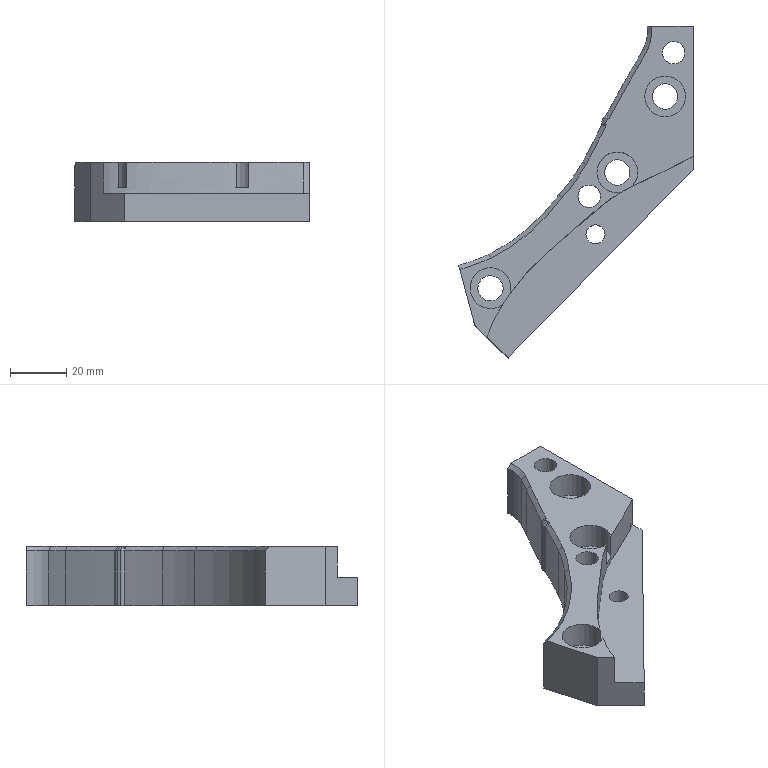Part | NX | features 23 2 | 1 solid | 43 faces | box 83.342 x 117.885 x 21 mm | volume 54365 mm3 | cylinder 18 | plane 13 | cone 10 | spline 2 | commonest cylinder face diameters 9 x3 14.5 x3 4.4 x2 8.001 x2 6.8 x1 28.064 x1